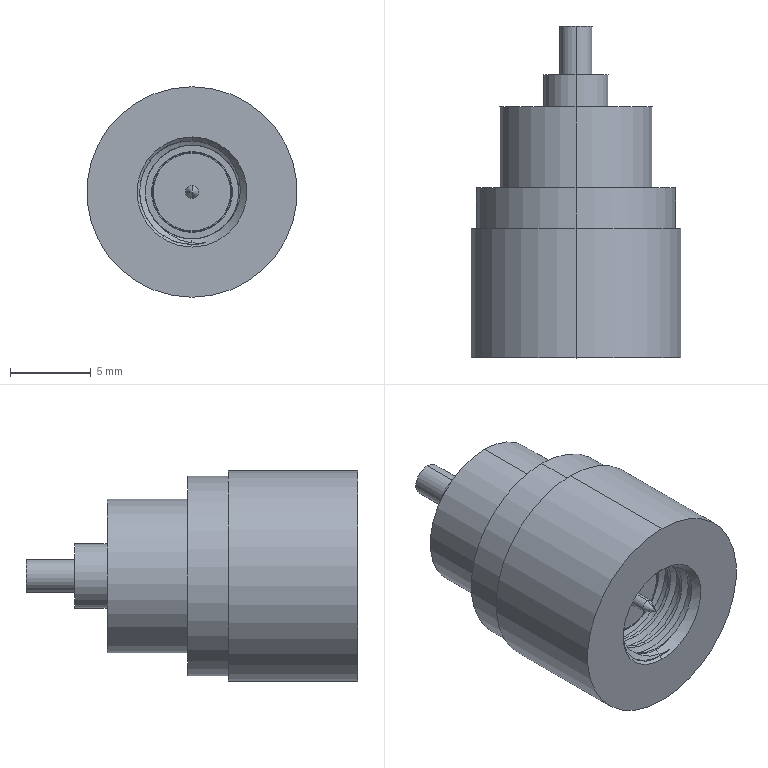Part | SolidWorks | features Chamfer 1, Helix 1, Revolution 1, SweepCut 1 | 1 solid | 54 faces | box 13 x 20.5 x 13 mm | volume 1624 mm3 | cylinder 33 | plane 12 | cone 5 | spline 4 | commonest cylinder face diameters 5.8 x13 0.8 x2 1 x2 2 x2 4 x2 4.807 x2